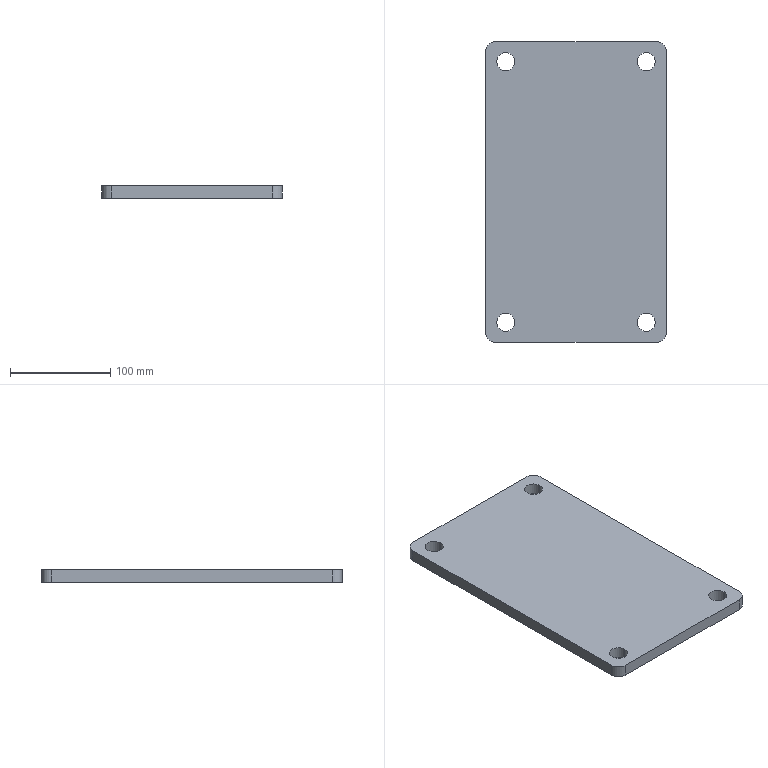Part | SolidWorks | features Extrusion 1, ICE 1 | 1 solid | 18 faces | box 180 x 300 x 12 mm | volume 634755 mm3 | cylinder 12 | plane 6 | commonest cylinder face diameters 18 x8 20 x4
STEP:
#1=CARTESIAN_POINT('',(61.,130.,-6.));
#2=VERTEX_POINT('',#1);
#3=CARTESIAN_POINT('',(79.,130.,-6.));
#4=VERTEX_POINT('',#3);
#5=CARTESIAN_POINT('',(70.,130.,-6.));
#6=DIRECTION('',(0.,0.,1.));
#7=DIRECTION('',(1.,0.,0.));
#8=AXIS2_PLACEMENT_3D('',#5,#6,#7);
#9=CIRCLE('',#8,9.);
#10=EDGE_CURVE('',#2,#4,#9,.T.);
#11=ORIENTED_EDGE('',*,*,#10,.F.);
#12=CARTESIAN_POINT('',(61.,130.,6.));
#13=VERTEX_POINT('',#12);
#14=CARTESIAN_POINT('',(61.,130.,-6.));
#15=DIRECTION('',(0.,0.,1.));
#16=VECTOR('',#15,1000.);
#17=LINE('',#14,#16);
#18=EDGE_CURVE('',#2,#13,#17,.T.);
#19=ORIENTED_EDGE('',*,*,#18,.T.);
#20=CARTESIAN_POINT('',(79.,130.,6.));
#21=VERTEX_POINT('',#20);
#22=CARTESIAN_POINT('',(70.,130.,6.));
#23=DIRECTION('',(0.,0.,1.));
#24=DIRECTION('',(1.,0.,0.));
#25=AXIS2_PLACEMENT_3D('',#22,#23,#24);
#26=CIRCLE('',#25,9.);
#27=EDGE_CURVE('',#13,#21,#26,.T.);
#28=ORIENTED_EDGE('',*,*,#27,.T.);
#29=CARTESIAN_POINT('',(79.,130.,-6.));
#30=DIRECTION('',(0.,0.,1.));
#31=VECTOR('',#30,1000.);
#32=LINE('',#29,#31);
#33=EDGE_CURVE('',#4,#21,#32,.T.);
#34=ORIENTED_EDGE('',*,*,#33,.F.);
#35=EDGE_LOOP('',(#11,#19,#28,#34));
#36=FACE_OUTER_BOUND('',#35,.T.);
#37=CARTESIAN_POINT('',(70.,130.,-6.));
#38=DIRECTION('',(0.,0.,1.));
#39=DIRECTION('',(1.,0.,0.));
#40=AXIS2_PLACEMENT_3D('',#37,#38,#39);
#41=CYLINDRICAL_SURFACE('',#40,9.);
#42=ADVANCED_FACE('',(#36),#41,.F.);
#43=CARTESIAN_POINT('',(-79.,130.,-6.));
#44=VERTEX_POINT('',#43);
#45=CARTESIAN_POINT('',(-61.,130.,-6.));
#46=VERTEX_POINT('',#45);
#47=CARTESIAN_POINT('',(-70.,130.,-6.));
#48=DIRECTION('',(0.,0.,1.));
#49=DIRECTION('',(1.,0.,0.));
#50=AXIS2_PLACEMENT_3D('',#47,#48,#49);
#51=CIRCLE('',#50,9.);
#52=EDGE_CURVE('',#44,#46,#51,.T.);
#53=ORIENTED_EDGE('',*,*,#52,.F.);
#54=CARTESIAN_POINT('',(-79.,130.,6.));
#55=VERTEX_POINT('',#54);
#56=CARTESIAN_POINT('',(-79.,130.,-6.));
#57=DIRECTION('',(0.,0.,1.));
#58=VECTOR('',#57,1000.);
#59=LINE('',#56,#58);
#60=EDGE_CURVE('',#44,#55,#59,.T.);
#61=ORIENTED_EDGE('',*,*,#60,.T.);
#62=CARTESIAN_POINT('',(-61.,130.,6.));
#63=VERTEX_POINT('',#62);
#64=CARTESIAN_POINT('',(-70.,130.,6.));
#65=DIRECTION('',(0.,0.,1.));
#66=DIRECTION('',(1.,0.,0.));
#67=AXIS2_PLACEMENT_3D('',#64,#65,#66);
#68=CIRCLE('',#67,9.);
#69=EDGE_CURVE('',#55,#63,#68,.T.);
#70=ORIENTED_EDGE('',*,*,#69,.T.);
#71=CARTESIAN_POINT('',(-61.,130.,-6.));
#72=DIRECTION('',(0.,0.,1.));
#73=VECTOR('',#72,1000.);
#74=LINE('',#71,#73);
#75=EDGE_CURVE('',#46,#63,#74,.T.);
#76=ORIENTED_EDGE('',*,*,#75,.F.);
#77=EDGE_LOOP('',(#53,#61,#70,#76));
#78=FACE_OUTER_BOUND('',#77,.T.);
#79=CARTESIAN_POINT('',(-70.,130.,-6.));
#80=DIRECTION('',(0.,0.,1.));
#81=DIRECTION('',(1.,0.,0.));
#82=AXIS2_PLACEMENT_3D('',#79,#80,#81);
#83=CYLINDRICAL_SURFACE('',#82,9.);
#84=ADVANCED_FACE('',(#78),#83,.F.);
#85=CARTESIAN_POINT('',(61.,-130.,-6.));
#86=VERTEX_POINT('',#85);
#87=CARTESIAN_POINT('',(79.,-130.,-6.));
#88=VERTEX_POINT('',#87);
#89=CARTESIAN_POINT('',(70.,-130.,-6.));
#90=DIRECTION('',(0.,0.,1.));
#91=DIRECTION('',(1.,0.,0.));
#92=AXIS2_PLACEMENT_3D('',#89,#90,#91);
#93=CIRCLE('',#92,9.);
#94=EDGE_CURVE('',#86,#88,#93,.T.);
#95=ORIENTED_EDGE('',*,*,#94,.F.);
#96=CARTESIAN_POINT('',(61.,-130.,6.));
#97=VERTEX_POINT('',#96);
#98=CARTESIAN_POINT('',(61.,-130.,-6.));
#99=DIRECTION('',(0.,0.,1.));
#100=VECTOR('',#99,1000.);
#101=LINE('',#98,#100);
#102=EDGE_CURVE('',#86,#97,#101,.T.);
#103=ORIENTED_EDGE('',*,*,#102,.T.);
#104=CARTESIAN_POINT('',(79.,-130.,6.));
#105=VERTEX_POINT('',#104);
#106=CARTESIAN_POINT('',(70.,-130.,6.));
#107=DIRECTION('',(0.,0.,1.));
#108=DIRECTION('',(1.,0.,0.));
#109=AXIS2_PLACEMENT_3D('',#106,#107,#108);
#110=CIRCLE('',#109,9.);
#111=EDGE_CURVE('',#97,#105,#110,.T.);
#112=ORIENTED_EDGE('',*,*,#111,.T.);
#113=CARTESIAN_POINT('',(79.,-130.,-6.));
#114=DIRECTION('',(0.,0.,1.));
#115=VECTOR('',#114,1000.);
#116=LINE('',#113,#115);
#117=EDGE_CURVE('',#88,#105,#116,.T.);
#118=ORIENTED_EDGE('',*,*,#117,.F.);
#119=EDGE_LOOP('',(#95,#103,#112,#118));
#120=FACE_OUTER_BOUND('',#119,.T.);
#121=CARTESIAN_POINT('',(70.,-130.,-6.));
#122=DIRECTION('',(0.,0.,1.));
#123=DIRECTION('',(1.,0.,0.));
#124=AXIS2_PLACEMENT_3D('',#121,#122,#123);
#125=CYLINDRICAL_SURFACE('',#124,9.);
#126=ADVANCED_FACE('',(#120),#125,.F.);
#127=CARTESIAN_POINT('',(-79.,-130.,-6.));
#128=VERTEX_POINT('',#127);
#129=CARTESIAN_POINT('',(-61.,-130.,-6.));
#130=VERTEX_POINT('',#129);
#131=CARTESIAN_POINT('',(-70.,-130.,-6.));
#132=DIRECTION('',(0.,0.,1.));
#133=DIRECTION('',(1.,0.,0.));
#134=AXIS2_PLACEMENT_3D('',#131,#132,#133);
#135=CIRCLE('',#134,9.);
#136=EDGE_CURVE('',#128,#130,#135,.T.);
#137=ORIENTED_EDGE('',*,*,#136,.F.);
#138=CARTESIAN_POINT('',(-79.,-130.,6.));
#139=VERTEX_POINT('',#138);
#140=CARTESIAN_POINT('',(-79.,-130.,-6.));
#141=DIRECTION('',(0.,0.,1.));
#142=VECTOR('',#141,1000.);
#143=LINE('',#140,#142);
#144=EDGE_CURVE('',#128,#139,#143,.T.);
#145=ORIENTED_EDGE('',*,*,#144,.T.);
#146=CARTESIAN_POINT('',(-61.,-130.,6.));
#147=VERTEX_POINT('',#146);
#148=CARTESIAN_POINT('',(-70.,-130.,6.));
#149=DIRECTION('',(0.,0.,1.));
#150=DIRECTION('',(1.,0.,0.));
#151=AXIS2_PLACEMENT_3D('',#148,#149,#150);
#152=CIRCLE('',#151,9.);
#153=EDGE_CURVE('',#139,#147,#152,.T.);
#154=ORIENTED_EDGE('',*,*,#153,.T.);
#155=CARTESIAN_POINT('',(-61.,-130.,-6.));
#156=DIRECTION('',(0.,0.,1.));
#157=VECTOR('',#156,1000.);
#158=LINE('',#155,#157);
#159=EDGE_CURVE('',#130,#147,#158,.T.);
#160=ORIENTED_EDGE('',*,*,#159,.F.);
#161=EDGE_LOOP('',(#137,#145,#154,#160));
#162=FACE_OUTER_BOUND('',#161,.T.);
#163=CARTESIAN_POINT('',(-70.,-130.,-6.));
#164=DIRECTION('',(0.,0.,1.));
#165=DIRECTION('',(1.,0.,0.));
#166=AXIS2_PLACEMENT_3D('',#163,#164,#165);
#167=CYLINDRICAL_SURFACE('',#166,9.);
#168=ADVANCED_FACE('',(#162),#167,.F.);
#169=CARTESIAN_POINT('',(-80.,150.,-6.));
#170=VERTEX_POINT('',#169);
#171=CARTESIAN_POINT('',(-90.,140.,-6.));
#172=VERTEX_POINT('',#171);
#173=CARTESIAN_POINT('',(-80.,140.,-6.));
#174=DIRECTION('',(0.,0.,1.));
#175=DIRECTION('',(1.,0.,0.));
#176=AXIS2_PLACEMENT_3D('',#173,#174,#175);
#177=CIRCLE('',#176,10.);
#178=EDGE_CURVE('',#170,#172,#177,.T.);
#179=ORIENTED_EDGE('',*,*,#178,.T.);
#180=CARTESIAN_POINT('',(-90.,140.,6.));
#181=VERTEX_POINT('',#180);
#182=CARTESIAN_POINT('',(-90.,140.,6.));
#183=DIRECTION('',(0.,0.,-1.));
#184=VECTOR('',#183,1000.);
#185=LINE('',#182,#184);
#186=EDGE_CURVE('',#181,#172,#185,.T.);
#187=ORIENTED_EDGE('',*,*,#186,.F.);
#188=CARTESIAN_POINT('',(-80.,150.,6.));
#189=VERTEX_POINT('',#188);
#190=CARTESIAN_POINT('',(-80.,140.,6.));
#191=DIRECTION('',(0.,0.,1.));
#192=DIRECTION('',(1.,0.,0.));
#193=AXIS2_PLACEMENT_3D('',#190,#191,#192);
#194=CIRCLE('',#193,10.);
#195=EDGE_CURVE('',#189,#181,#194,.T.);
#196=ORIENTED_EDGE('',*,*,#195,.F.);
#197=CARTESIAN_POINT('',(-80.,150.,6.));
#198=DIRECTION('',(0.,0.,-1.));
#199=VECTOR('',#198,1000.);
#200=LINE('',#197,#199);
#201=EDGE_CURVE('',#189,#170,#200,.T.);
#202=ORIENTED_EDGE('',*,*,#201,.T.);
#203=EDGE_LOOP('',(#179,#187,#196,#202));
#204=FACE_OUTER_BOUND('',#203,.T.);
#205=CARTESIAN_POINT('',(-80.,140.,6.));
#206=DIRECTION('',(0.,0.,-1.));
#207=DIRECTION('',(-1.,0.,0.));
#208=AXIS2_PLACEMENT_3D('',#205,#206,#207);
#209=CYLINDRICAL_SURFACE('',#208,10.);
#210=ADVANCED_FACE('',(#204),#209,.T.);
#211=CARTESIAN_POINT('',(-90.,-140.,-6.));
#212=VERTEX_POINT('',#211);
#213=CARTESIAN_POINT('',(-90.,140.,-6.));
#214=DIRECTION('',(0.,-1.,0.));
#215=VECTOR('',#214,1000.);
#216=LINE('',#213,#215);
#217=EDGE_CURVE('',#172,#212,#216,.T.);
#218=ORIENTED_EDGE('',*,*,#217,.T.);
#219=CARTESIAN_POINT('',(-90.,-140.,6.));
#220=VERTEX_POINT('',#219);
#221=CARTESIAN_POINT('',(-90.,-140.,6.));
#222=DIRECTION('',(0.,0.,-1.));
#223=VECTOR('',#222,1000.);
#224=LINE('',#221,#223);
#225=EDGE_CURVE('',#220,#212,#224,.T.);
#226=ORIENTED_EDGE('',*,*,#225,.F.);
#227=CARTESIAN_POINT('',(-90.,140.,6.));
#228=DIRECTION('',(0.,-1.,0.));
#229=VECTOR('',#228,1000.);
#230=LINE('',#227,#229);
#231=EDGE_CURVE('',#181,#220,#230,.T.);
#232=ORIENTED_EDGE('',*,*,#231,.F.);
#233=ORIENTED_EDGE('',*,*,#186,.T.);
#234=EDGE_LOOP('',(#218,#226,#232,#233));
#235=FACE_OUTER_BOUND('',#234,.T.);
#236=CARTESIAN_POINT('',(-90.,140.,6.));
#237=DIRECTION('',(1.,0.,0.));
#238=DIRECTION('',(0.,1.,0.));
#239=AXIS2_PLACEMENT_3D('',#236,#237,#238);
#240=PLANE('',#239);
#241=ADVANCED_FACE('',(#235),#240,.F.);
#242=CARTESIAN_POINT('',(-80.,-150.,-6.));
#243=VERTEX_POINT('',#242);
#244=CARTESIAN_POINT('',(-80.,-140.,-6.));
#245=DIRECTION('',(0.,0.,1.));
#246=DIRECTION('',(1.,0.,0.));
#247=AXIS2_PLACEMENT_3D('',#244,#245,#246);
#248=CIRCLE('',#247,10.);
#249=EDGE_CURVE('',#212,#243,#248,.T.);
#250=ORIENTED_EDGE('',*,*,#249,.T.);
#251=CARTESIAN_POINT('',(-80.,-150.,6.));
#252=VERTEX_POINT('',#251);
#253=CARTESIAN_POINT('',(-80.,-150.,6.));
#254=DIRECTION('',(0.,0.,-1.));
#255=VECTOR('',#254,1000.);
#256=LINE('',#253,#255);
#257=EDGE_CURVE('',#252,#243,#256,.T.);
#258=ORIENTED_EDGE('',*,*,#257,.F.);
#259=CARTESIAN_POINT('',(-80.,-140.,6.));
#260=DIRECTION('',(0.,0.,1.));
#261=DIRECTION('',(1.,0.,0.));
#262=AXIS2_PLACEMENT_3D('',#259,#260,#261);
#263=CIRCLE('',#262,10.);
#264=EDGE_CURVE('',#220,#252,#263,.T.);
#265=ORIENTED_EDGE('',*,*,#264,.F.);
#266=ORIENTED_EDGE('',*,*,#225,.T.);
#267=EDGE_LOOP('',(#250,#258,#265,#266));
#268=FACE_OUTER_BOUND('',#267,.T.);
#269=CARTESIAN_POINT('',(-80.,-140.,6.));
#270=DIRECTION('',(0.,0.,-1.));
#271=DIRECTION('',(-1.,0.,0.));
#272=AXIS2_PLACEMENT_3D('',#269,#270,#271);
#273=CYLINDRICAL_SURFACE('',#272,10.);
#274=ADVANCED_FACE('',(#268),#273,.T.);
#275=CARTESIAN_POINT('',(80.,-150.,-6.));
#276=VERTEX_POINT('',#275);
#277=CARTESIAN_POINT('',(-80.,-150.,-6.));
#278=DIRECTION('',(1.,0.,0.));
#279=VECTOR('',#278,1000.);
#280=LINE('',#277,#279);
#281=EDGE_CURVE('',#243,#276,#280,.T.);
#282=ORIENTED_EDGE('',*,*,#281,.T.);
#283=CARTESIAN_POINT('',(80.,-150.,6.));
#284=VERTEX_POINT('',#283);
#285=CARTESIAN_POINT('',(80.,-150.,6.));
#286=DIRECTION('',(0.,0.,-1.));
#287=VECTOR('',#286,1000.);
#288=LINE('',#285,#287);
#289=EDGE_CURVE('',#284,#276,#288,.T.);
#290=ORIENTED_EDGE('',*,*,#289,.F.);
#291=CARTESIAN_POINT('',(-80.,-150.,6.));
#292=DIRECTION('',(1.,0.,0.));
#293=VECTOR('',#292,1000.);
#294=LINE('',#291,#293);
#295=EDGE_CURVE('',#252,#284,#294,.T.);
#296=ORIENTED_EDGE('',*,*,#295,.F.);
#297=ORIENTED_EDGE('',*,*,#257,.T.);
#298=EDGE_LOOP('',(#282,#290,#296,#297));
#299=FACE_OUTER_BOUND('',#298,.T.);
#300=CARTESIAN_POINT('',(-80.,-150.,6.));
#301=DIRECTION('',(0.,1.,0.));
#302=DIRECTION('',(0.,0.,1.));
#303=AXIS2_PLACEMENT_3D('',#300,#301,#302);
#304=PLANE('',#303);
#305=ADVANCED_FACE('',(#299),#304,.F.);
#306=CARTESIAN_POINT('',(90.,-140.,-6.));
#307=VERTEX_POINT('',#306);
#308=CARTESIAN_POINT('',(80.,-140.,-6.));
#309=DIRECTION('',(0.,0.,1.));
#310=DIRECTION('',(1.,0.,0.));
#311=AXIS2_PLACEMENT_3D('',#308,#309,#310);
#312=CIRCLE('',#311,10.);
#313=EDGE_CURVE('',#276,#307,#312,.T.);
#314=ORIENTED_EDGE('',*,*,#313,.T.);
#315=CARTESIAN_POINT('',(90.,-140.,6.));
#316=VERTEX_POINT('',#315);
#317=CARTESIAN_POINT('',(90.,-140.,6.));
#318=DIRECTION('',(0.,0.,-1.));
#319=VECTOR('',#318,1000.);
#320=LINE('',#317,#319);
#321=EDGE_CURVE('',#316,#307,#320,.T.);
#322=ORIENTED_EDGE('',*,*,#321,.F.);
#323=CARTESIAN_POINT('',(80.,-140.,6.));
#324=DIRECTION('',(0.,0.,1.));
#325=DIRECTION('',(1.,0.,0.));
#326=AXIS2_PLACEMENT_3D('',#323,#324,#325);
#327=CIRCLE('',#326,10.);
#328=EDGE_CURVE('',#284,#316,#327,.T.);
#329=ORIENTED_EDGE('',*,*,#328,.F.);
#330=ORIENTED_EDGE('',*,*,#289,.T.);
#331=EDGE_LOOP('',(#314,#322,#329,#330));
#332=FACE_OUTER_BOUND('',#331,.T.);
#333=CARTESIAN_POINT('',(80.,-140.,6.));
#334=DIRECTION('',(0.,0.,-1.));
#335=DIRECTION('',(-1.,0.,0.));
#336=AXIS2_PLACEMENT_3D('',#333,#334,#335);
#337=CYLINDRICAL_SURFACE('',#336,10.);
#338=ADVANCED_FACE('',(#332),#337,.T.);
#339=CARTESIAN_POINT('',(90.,140.,-6.));
#340=VERTEX_POINT('',#339);
#341=CARTESIAN_POINT('',(90.,-140.,-6.));
#342=DIRECTION('',(0.,1.,0.));
#343=VECTOR('',#342,1000.);
#344=LINE('',#341,#343);
#345=EDGE_CURVE('',#307,#340,#344,.T.);
#346=ORIENTED_EDGE('',*,*,#345,.T.);
#347=CARTESIAN_POINT('',(90.,140.,6.));
#348=VERTEX_POINT('',#347);
#349=CARTESIAN_POINT('',(90.,140.,6.));
#350=DIRECTION('',(0.,0.,-1.));
#351=VECTOR('',#350,1000.);
#352=LINE('',#349,#351);
#353=EDGE_CURVE('',#348,#340,#352,.T.);
#354=ORIENTED_EDGE('',*,*,#353,.F.);
#355=CARTESIAN_POINT('',(90.,-140.,6.));
#356=DIRECTION('',(0.,1.,0.));
#357=VECTOR('',#356,1000.);
#358=LINE('',#355,#357);
#359=EDGE_CURVE('',#316,#348,#358,.T.);
#360=ORIENTED_EDGE('',*,*,#359,.F.);
#361=ORIENTED_EDGE('',*,*,#321,.T.);
#362=EDGE_LOOP('',(#346,#354,#360,#361));
#363=FACE_OUTER_BOUND('',#362,.T.);
#364=CARTESIAN_POINT('',(90.,-140.,6.));
#365=DIRECTION('',(-1.,0.,0.));
#366=DIRECTION('',(0.,0.,1.));
#367=AXIS2_PLACEMENT_3D('',#364,#365,#366);
#368=PLANE('',#367);
#369=ADVANCED_FACE('',(#363),#368,.F.);
#370=CARTESIAN_POINT('',(80.,150.,-6.));
#371=VERTEX_POINT('',#370);
#372=CARTESIAN_POINT('',(80.,140.,-6.));
#373=DIRECTION('',(0.,0.,1.));
#374=DIRECTION('',(1.,0.,0.));
#375=AXIS2_PLACEMENT_3D('',#372,#373,#374);
#376=CIRCLE('',#375,10.);
#377=EDGE_CURVE('',#340,#371,#376,.T.);
#378=ORIENTED_EDGE('',*,*,#377,.T.);
#379=CARTESIAN_POINT('',(80.,150.,6.));
#380=VERTEX_POINT('',#379);
#381=CARTESIAN_POINT('',(80.,150.,6.));
#382=DIRECTION('',(0.,0.,-1.));
#383=VECTOR('',#382,1000.);
#384=LINE('',#381,#383);
#385=EDGE_CURVE('',#380,#371,#384,.T.);
#386=ORIENTED_EDGE('',*,*,#385,.F.);
#387=CARTESIAN_POINT('',(80.,140.,6.));
#388=DIRECTION('',(0.,0.,1.));
#389=DIRECTION('',(1.,0.,0.));
#390=AXIS2_PLACEMENT_3D('',#387,#388,#389);
#391=CIRCLE('',#390,10.);
#392=EDGE_CURVE('',#348,#380,#391,.T.);
#393=ORIENTED_EDGE('',*,*,#392,.F.);
#394=ORIENTED_EDGE('',*,*,#353,.T.);
#395=EDGE_LOOP('',(#378,#386,#393,#394));
#396=FACE_OUTER_BOUND('',#395,.T.);
#397=CARTESIAN_POINT('',(80.,140.,6.));
#398=DIRECTION('',(0.,0.,-1.));
#399=DIRECTION('',(-1.,0.,0.));
#400=AXIS2_PLACEMENT_3D('',#397,#398,#399);
#401=CYLINDRICAL_SURFACE('',#400,10.);
#402=ADVANCED_FACE('',(#396),#401,.T.);
#403=CARTESIAN_POINT('',(80.,150.,-6.));
#404=DIRECTION('',(-1.,0.,0.));
#405=VECTOR('',#404,1000.);
#406=LINE('',#403,#405);
#407=EDGE_CURVE('',#371,#170,#406,.T.);
#408=ORIENTED_EDGE('',*,*,#407,.T.);
#409=ORIENTED_EDGE('',*,*,#201,.F.);
#410=CARTESIAN_POINT('',(80.,150.,6.));
#411=DIRECTION('',(-1.,0.,0.));
#412=VECTOR('',#411,1000.);
#413=LINE('',#410,#412);
#414=EDGE_CURVE('',#380,#189,#413,.T.);
#415=ORIENTED_EDGE('',*,*,#414,.F.);
#416=ORIENTED_EDGE('',*,*,#385,.T.);
#417=EDGE_LOOP('',(#408,#409,#415,#416));
#418=FACE_OUTER_BOUND('',#417,.T.);
#419=CARTESIAN_POINT('',(80.,150.,6.));
#420=DIRECTION('',(0.,-1.,0.));
#421=DIRECTION('',(0.,0.,-1.));
#422=AXIS2_PLACEMENT_3D('',#419,#420,#421);
#423=PLANE('',#422);
#424=ADVANCED_FACE('',(#418),#423,.F.);
#425=CARTESIAN_POINT('',(70.,130.,6.));
#426=DIRECTION('',(0.,0.,1.));
#427=DIRECTION('',(1.,0.,0.));
#428=AXIS2_PLACEMENT_3D('',#425,#426,#427);
#429=CIRCLE('',#428,9.);
#430=EDGE_CURVE('',#21,#13,#429,.T.);
#431=ORIENTED_EDGE('',*,*,#430,.F.);
#432=ORIENTED_EDGE('',*,*,#27,.F.);
#433=EDGE_LOOP('',(#431,#432));
#434=FACE_BOUND('',#433,.T.);
#435=CARTESIAN_POINT('',(-70.,130.,6.));
#436=DIRECTION('',(0.,0.,1.));
#437=DIRECTION('',(1.,0.,0.));
#438=AXIS2_PLACEMENT_3D('',#435,#436,#437);
#439=CIRCLE('',#438,9.);
#440=EDGE_CURVE('',#63,#55,#439,.T.);
#441=ORIENTED_EDGE('',*,*,#440,.F.);
#442=ORIENTED_EDGE('',*,*,#69,.F.);
#443=EDGE_LOOP('',(#441,#442));
#444=FACE_BOUND('',#443,.T.);
#445=CARTESIAN_POINT('',(70.,-130.,6.));
#446=DIRECTION('',(0.,0.,1.));
#447=DIRECTION('',(1.,0.,0.));
#448=AXIS2_PLACEMENT_3D('',#445,#446,#447);
#449=CIRCLE('',#448,9.);
#450=EDGE_CURVE('',#105,#97,#449,.T.);
#451=ORIENTED_EDGE('',*,*,#450,.F.);
#452=ORIENTED_EDGE('',*,*,#111,.F.);
#453=EDGE_LOOP('',(#451,#452));
#454=FACE_BOUND('',#453,.T.);
#455=CARTESIAN_POINT('',(-70.,-130.,6.));
#456=DIRECTION('',(0.,0.,1.));
#457=DIRECTION('',(1.,0.,0.));
#458=AXIS2_PLACEMENT_3D('',#455,#456,#457);
#459=CIRCLE('',#458,9.);
#460=EDGE_CURVE('',#147,#139,#459,.T.);
#461=ORIENTED_EDGE('',*,*,#460,.F.);
#462=ORIENTED_EDGE('',*,*,#153,.F.);
#463=EDGE_LOOP('',(#461,#462));
#464=FACE_BOUND('',#463,.T.);
#465=ORIENTED_EDGE('',*,*,#195,.T.);
#466=ORIENTED_EDGE('',*,*,#231,.T.);
#467=ORIENTED_EDGE('',*,*,#264,.T.);
#468=ORIENTED_EDGE('',*,*,#295,.T.);
#469=ORIENTED_EDGE('',*,*,#328,.T.);
#470=ORIENTED_EDGE('',*,*,#359,.T.);
#471=ORIENTED_EDGE('',*,*,#392,.T.);
#472=ORIENTED_EDGE('',*,*,#414,.T.);
#473=EDGE_LOOP('',(#465,#466,#467,#468,#469,#470,#471,#472));
#474=FACE_OUTER_BOUND('',#473,.T.);
#475=CARTESIAN_POINT('',(-80.,140.,6.));
#476=DIRECTION('',(0.,0.,1.));
#477=DIRECTION('',(1.,0.,0.));
#478=AXIS2_PLACEMENT_3D('',#475,#476,#477);
#479=PLANE('',#478);
#480=ADVANCED_FACE('',(#434,#444,#454,#464,#474),#479,.T.);
#481=CARTESIAN_POINT('',(70.,130.,-6.));
#482=DIRECTION('',(0.,0.,1.));
#483=DIRECTION('',(1.,0.,0.));
#484=AXIS2_PLACEMENT_3D('',#481,#482,#483);
#485=CIRCLE('',#484,9.);
#486=EDGE_CURVE('',#4,#2,#485,.T.);
#487=ORIENTED_EDGE('',*,*,#486,.T.);
#488=ORIENTED_EDGE('',*,*,#10,.T.);
#489=EDGE_LOOP('',(#487,#488));
#490=FACE_BOUND('',#489,.T.);
#491=CARTESIAN_POINT('',(-70.,130.,-6.));
#492=DIRECTION('',(0.,0.,1.));
#493=DIRECTION('',(1.,0.,0.));
#494=AXIS2_PLACEMENT_3D('',#491,#492,#493);
#495=CIRCLE('',#494,9.);
#496=EDGE_CURVE('',#46,#44,#495,.T.);
#497=ORIENTED_EDGE('',*,*,#496,.T.);
#498=ORIENTED_EDGE('',*,*,#52,.T.);
#499=EDGE_LOOP('',(#497,#498));
#500=FACE_BOUND('',#499,.T.);
#501=CARTESIAN_POINT('',(70.,-130.,-6.));
#502=DIRECTION('',(0.,0.,1.));
#503=DIRECTION('',(1.,0.,0.));
#504=AXIS2_PLACEMENT_3D('',#501,#502,#503);
#505=CIRCLE('',#504,9.);
#506=EDGE_CURVE('',#88,#86,#505,.T.);
#507=ORIENTED_EDGE('',*,*,#506,.T.);
#508=ORIENTED_EDGE('',*,*,#94,.T.);
#509=EDGE_LOOP('',(#507,#508));
#510=FACE_BOUND('',#509,.T.);
#511=CARTESIAN_POINT('',(-70.,-130.,-6.));
#512=DIRECTION('',(0.,0.,1.));
#513=DIRECTION('',(1.,0.,0.));
#514=AXIS2_PLACEMENT_3D('',#511,#512,#513);
#515=CIRCLE('',#514,9.);
#516=EDGE_CURVE('',#130,#128,#515,.T.);
#517=ORIENTED_EDGE('',*,*,#516,.T.);
#518=ORIENTED_EDGE('',*,*,#136,.T.);
#519=EDGE_LOOP('',(#517,#518));
#520=FACE_BOUND('',#519,.T.);
#521=ORIENTED_EDGE('',*,*,#178,.F.);
#522=ORIENTED_EDGE('',*,*,#407,.F.);
#523=ORIENTED_EDGE('',*,*,#377,.F.);
#524=ORIENTED_EDGE('',*,*,#345,.F.);
#525=ORIENTED_EDGE('',*,*,#313,.F.);
#526=ORIENTED_EDGE('',*,*,#281,.F.);
#527=ORIENTED_EDGE('',*,*,#249,.F.);
#528=ORIENTED_EDGE('',*,*,#217,.F.);
#529=EDGE_LOOP('',(#521,#522,#523,#524,#525,#526,#527,#528));
#530=FACE_OUTER_BOUND('',#529,.T.);
#531=CARTESIAN_POINT('',(-80.,140.,-6.));
#532=DIRECTION('',(0.,0.,1.));
#533=DIRECTION('',(1.,0.,0.));
#534=AXIS2_PLACEMENT_3D('',#531,#532,#533);
#535=PLANE('',#534);
#536=ADVANCED_FACE('',(#490,#500,#510,#520,#530),#535,.F.);
#537=ORIENTED_EDGE('',*,*,#144,.F.);
#538=ORIENTED_EDGE('',*,*,#516,.F.);
#539=ORIENTED_EDGE('',*,*,#159,.T.);
#540=ORIENTED_EDGE('',*,*,#460,.T.);
#541=EDGE_LOOP('',(#537,#538,#539,#540));
#542=FACE_OUTER_BOUND('',#541,.T.);
#543=CARTESIAN_POINT('',(-70.,-130.,-6.));
#544=DIRECTION('',(0.,0.,1.));
#545=DIRECTION('',(1.,0.,0.));
#546=AXIS2_PLACEMENT_3D('',#543,#544,#545);
#547=CYLINDRICAL_SURFACE('',#546,9.);
#548=ADVANCED_FACE('',(#542),#547,.F.);
#549=ORIENTED_EDGE('',*,*,#102,.F.);
#550=ORIENTED_EDGE('',*,*,#506,.F.);
#551=ORIENTED_EDGE('',*,*,#117,.T.);
#552=ORIENTED_EDGE('',*,*,#450,.T.);
#553=EDGE_LOOP('',(#549,#550,#551,#552));
#554=FACE_OUTER_BOUND('',#553,.T.);
#555=CARTESIAN_POINT('',(70.,-130.,-6.));
#556=DIRECTION('',(0.,0.,1.));
#557=DIRECTION('',(1.,0.,0.));
#558=AXIS2_PLACEMENT_3D('',#555,#556,#557);
#559=CYLINDRICAL_SURFACE('',#558,9.);
#560=ADVANCED_FACE('',(#554),#559,.F.);
#561=ORIENTED_EDGE('',*,*,#60,.F.);
#562=ORIENTED_EDGE('',*,*,#496,.F.);
#563=ORIENTED_EDGE('',*,*,#75,.T.);
#564=ORIENTED_EDGE('',*,*,#440,.T.);
#565=EDGE_LOOP('',(#561,#562,#563,#564));
#566=FACE_OUTER_BOUND('',#565,.T.);
#567=CARTESIAN_POINT('',(-70.,130.,-6.));
#568=DIRECTION('',(0.,0.,1.));
#569=DIRECTION('',(1.,0.,0.));
#570=AXIS2_PLACEMENT_3D('',#567,#568,#569);
#571=CYLINDRICAL_SURFACE('',#570,9.);
#572=ADVANCED_FACE('',(#566),#571,.F.);
#573=ORIENTED_EDGE('',*,*,#18,.F.);
#574=ORIENTED_EDGE('',*,*,#486,.F.);
#575=ORIENTED_EDGE('',*,*,#33,.T.);
#576=ORIENTED_EDGE('',*,*,#430,.T.);
#577=EDGE_LOOP('',(#573,#574,#575,#576));
#578=FACE_OUTER_BOUND('',#577,.T.);
#579=CARTESIAN_POINT('',(70.,130.,-6.));
#580=DIRECTION('',(0.,0.,1.));
#581=DIRECTION('',(1.,0.,0.));
#582=AXIS2_PLACEMENT_3D('',#579,#580,#581);
#583=CYLINDRICAL_SURFACE('',#582,9.);
#584=ADVANCED_FACE('',(#578),#583,.F.);
#585=CLOSED_SHELL('',(#42,#84,#126,#168,#210,#241,#274,#305,#338,#369,#402,#424,#480,#536,#548,#560,#572,#584));
#586=MANIFOLD_SOLID_BREP('',#585);
#587=CARTESIAN_POINT('',(0.,0.,0.));
#588=DIRECTION('',(0.,0.,1.));
#589=DIRECTION('',(1.,0.,0.));
#590=AXIS2_PLACEMENT_3D('',#587,#588,#589);
#591=(LENGTH_UNIT()NAMED_UNIT(*)SI_UNIT(.MILLI.,.METRE.));
#592=UNCERTAINTY_MEASURE_WITH_UNIT(LENGTH_MEASURE(0.00001),#591,'','');
#593=(NAMED_UNIT(*)PLANE_ANGLE_UNIT()SI_UNIT($,.RADIAN.));
#594=(NAMED_UNIT(*)SI_UNIT($,.STERADIAN.)SOLID_ANGLE_UNIT());
#595=(GEOMETRIC_REPRESENTATION_CONTEXT(3)GLOBAL_UNCERTAINTY_ASSIGNED_CONTEXT((#592))GLOBAL_UNIT_ASSIGNED_CONTEXT((#591,#593,#594))REPRESENTATION_CONTEXT('',''));
#596=ADVANCED_BREP_SHAPE_REPRESENTATION('',(#586,#590),#595);